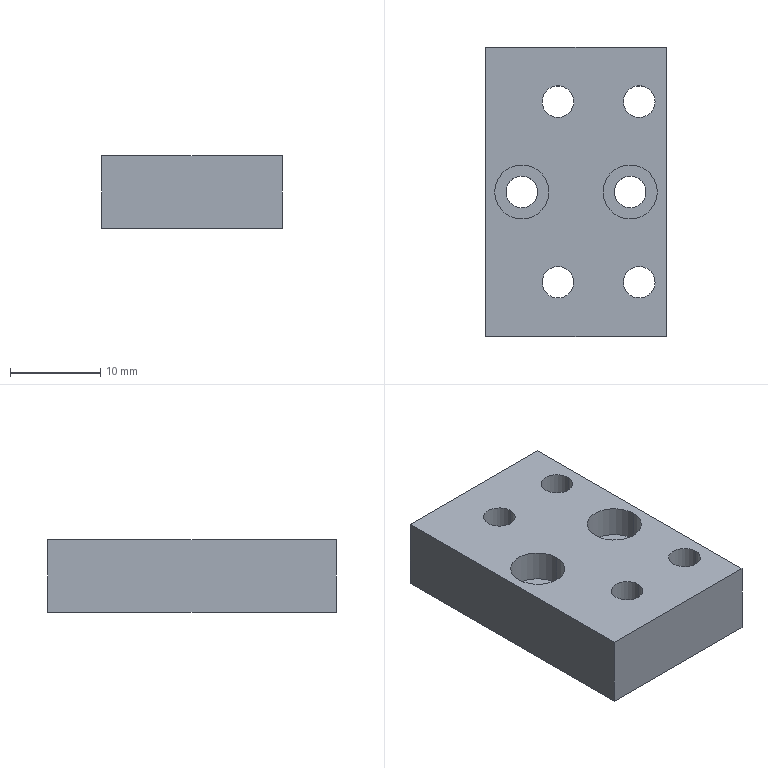Part | STEP file | Gripper cylinder connecting plate | 1 solid | 36 faces | box 20 x 32 x 8 mm | volume 4330 mm3 | cylinder 24 | plane 12 | commonest cylinder face diameters 3.5 x12 5.5 x8 6 x4